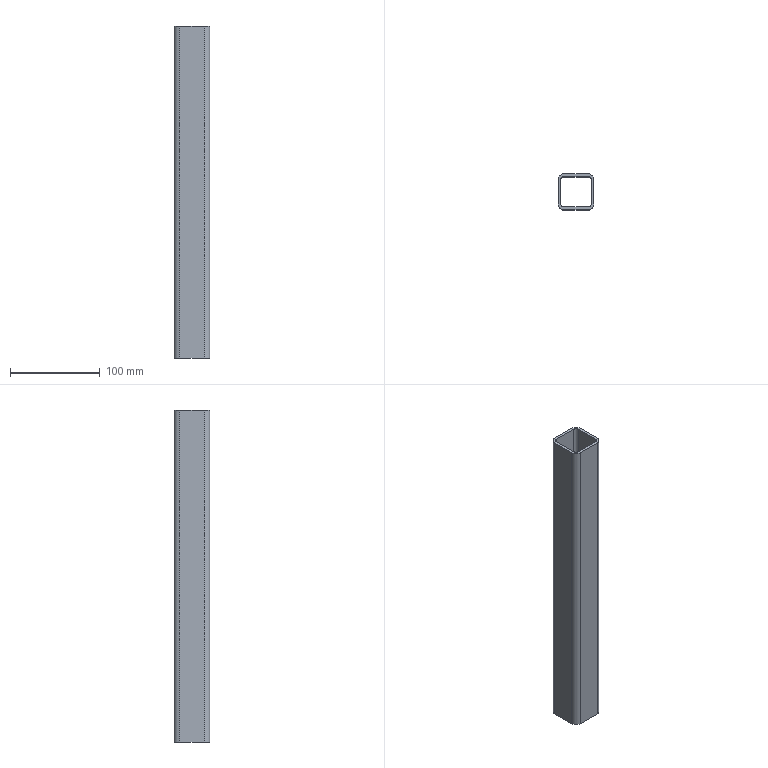Part | STEP file | 2 | 1 solid | 18 faces | box 40 x 40 x 370 mm | volume 154561 mm3 | plane 10 | cylinder 8 | commonest cylinder face diameters 7.2 x4 13.2 x4
STEP:
#1=CARTESIAN_POINT('',(0.,0.,0.));
#2=DIRECTION('',(0.,0.,1.));
#3=DIRECTION('',(1.,0.,0.));
#4=AXIS2_PLACEMENT_3D('',#1,#2,#3);
#5=CARTESIAN_POINT('',(-13.4,-17.,370.));
#6=VERTEX_POINT('',#5);
#7=CARTESIAN_POINT('',(13.4,-17.,370.));
#8=VERTEX_POINT('',#7);
#9=CARTESIAN_POINT('',(6.7,-17.,370.));
#10=DIRECTION('',(1.,0.,0.));
#11=VECTOR('',#10,1.);
#12=LINE('',#9,#11);
#13=CARTESIAN_POINT('',(13.4,-17.,0.));
#14=DIRECTION('',(0.,-1.,0.));
#15=DIRECTION('',(0.,0.,-1.));
#16=AXIS2_PLACEMENT_3D('',#13,#14,#15);
#17=PLANE('',#16);
#18=CARTESIAN_POINT('',(-370.,-6.7));
#19=DIRECTION('',(0.,1.));
#20=VECTOR('',#19,1.);
#21=LINE('',#18,#20);
#22=(GEOMETRIC_REPRESENTATION_CONTEXT(2)PARAMETRIC_REPRESENTATION_CONTEXT()REPRESENTATION_CONTEXT('',''));
#23=DEFINITIONAL_REPRESENTATION('',(#21),#22);
#24=PCURVE('',#17,#23);
#25=CARTESIAN_POINT('',(0.,0.,370.));
#26=DIRECTION('',(0.,0.,1.));
#27=DIRECTION('',(1.,0.,0.));
#28=AXIS2_PLACEMENT_3D('',#25,#26,#27);
#29=PLANE('',#28);
#30=CARTESIAN_POINT('',(6.7,-17.));
#31=DIRECTION('',(1.,0.));
#32=VECTOR('',#31,1.);
#33=LINE('',#30,#32);
#34=(GEOMETRIC_REPRESENTATION_CONTEXT(2)PARAMETRIC_REPRESENTATION_CONTEXT()REPRESENTATION_CONTEXT('',''));
#35=DEFINITIONAL_REPRESENTATION('',(#33),#34);
#36=PCURVE('',#29,#35);
#37=SURFACE_CURVE('',#12,(#24,#36),.PCURVE_S1.);
#38=EDGE_CURVE('',#6,#8,#37,.T.);
#39=ORIENTED_EDGE('',*,*,#38,.T.);
#40=CARTESIAN_POINT('',(13.4,-17.,0.));
#41=VERTEX_POINT('',#40);
#42=CARTESIAN_POINT('',(13.4,-17.,0.));
#43=DIRECTION('',(0.,0.,1.));
#44=VECTOR('',#43,1.);
#45=LINE('',#42,#44);
#46=CARTESIAN_POINT('',(0.,0.));
#47=DIRECTION('',(-1.,0.));
#48=VECTOR('',#47,1.);
#49=LINE('',#46,#48);
#50=(GEOMETRIC_REPRESENTATION_CONTEXT(2)PARAMETRIC_REPRESENTATION_CONTEXT()REPRESENTATION_CONTEXT('',''));
#51=DEFINITIONAL_REPRESENTATION('',(#49),#50);
#52=PCURVE('',#17,#51);
#53=CARTESIAN_POINT('',(13.4,-13.4,0.));
#54=DIRECTION('',(0.,0.,1.));
#55=DIRECTION('',(0.,1.,0.));
#56=AXIS2_PLACEMENT_3D('',#53,#54,#55);
#57=CYLINDRICAL_SURFACE('',#56,3.6);
#58=CARTESIAN_POINT('',(3.142,0.));
#59=DIRECTION('',(0.,1.));
#60=VECTOR('',#59,1.);
#61=LINE('',#58,#60);
#62=(GEOMETRIC_REPRESENTATION_CONTEXT(2)PARAMETRIC_REPRESENTATION_CONTEXT()REPRESENTATION_CONTEXT('',''));
#63=DEFINITIONAL_REPRESENTATION('',(#61),#62);
#64=PCURVE('',#57,#63);
#65=SURFACE_CURVE('',#45,(#52,#64),.PCURVE_S1.);
#66=EDGE_CURVE('',#41,#8,#65,.T.);
#67=ORIENTED_EDGE('',*,*,#66,.F.);
#68=CARTESIAN_POINT('',(-13.4,-17.,0.));
#69=VERTEX_POINT('',#68);
#70=CARTESIAN_POINT('',(6.7,-17.,0.));
#71=DIRECTION('',(1.,0.,0.));
#72=VECTOR('',#71,1.);
#73=LINE('',#70,#72);
#74=CARTESIAN_POINT('',(0.,-6.7));
#75=DIRECTION('',(0.,1.));
#76=VECTOR('',#75,1.);
#77=LINE('',#74,#76);
#78=(GEOMETRIC_REPRESENTATION_CONTEXT(2)PARAMETRIC_REPRESENTATION_CONTEXT()REPRESENTATION_CONTEXT('',''));
#79=DEFINITIONAL_REPRESENTATION('',(#77),#78);
#80=PCURVE('',#17,#79);
#81=CARTESIAN_POINT('',(0.,0.,0.));
#82=DIRECTION('',(0.,0.,1.));
#83=DIRECTION('',(1.,0.,0.));
#84=AXIS2_PLACEMENT_3D('',#81,#82,#83);
#85=PLANE('',#84);
#86=CARTESIAN_POINT('',(6.7,-17.));
#87=DIRECTION('',(1.,0.));
#88=VECTOR('',#87,1.);
#89=LINE('',#86,#88);
#90=(GEOMETRIC_REPRESENTATION_CONTEXT(2)PARAMETRIC_REPRESENTATION_CONTEXT()REPRESENTATION_CONTEXT('',''));
#91=DEFINITIONAL_REPRESENTATION('',(#89),#90);
#92=PCURVE('',#85,#91);
#93=SURFACE_CURVE('',#73,(#80,#92),.PCURVE_S1.);
#94=EDGE_CURVE('',#69,#41,#93,.T.);
#95=ORIENTED_EDGE('',*,*,#94,.F.);
#96=CARTESIAN_POINT('',(-13.4,-17.,0.));
#97=DIRECTION('',(0.,0.,1.));
#98=VECTOR('',#97,1.);
#99=LINE('',#96,#98);
#100=CARTESIAN_POINT('',(0.,-26.8));
#101=DIRECTION('',(-1.,0.));
#102=VECTOR('',#101,1.);
#103=LINE('',#100,#102);
#104=(GEOMETRIC_REPRESENTATION_CONTEXT(2)PARAMETRIC_REPRESENTATION_CONTEXT()REPRESENTATION_CONTEXT('',''));
#105=DEFINITIONAL_REPRESENTATION('',(#103),#104);
#106=PCURVE('',#17,#105);
#107=CARTESIAN_POINT('',(-13.4,-13.4,0.));
#108=DIRECTION('',(0.,0.,1.));
#109=DIRECTION('',(1.,0.,0.));
#110=AXIS2_PLACEMENT_3D('',#107,#108,#109);
#111=CYLINDRICAL_SURFACE('',#110,3.6);
#112=CARTESIAN_POINT('',(4.712,0.));
#113=DIRECTION('',(0.,1.));
#114=VECTOR('',#113,1.);
#115=LINE('',#112,#114);
#116=(GEOMETRIC_REPRESENTATION_CONTEXT(2)PARAMETRIC_REPRESENTATION_CONTEXT()REPRESENTATION_CONTEXT('',''));
#117=DEFINITIONAL_REPRESENTATION('',(#115),#116);
#118=PCURVE('',#111,#117);
#119=SURFACE_CURVE('',#99,(#106,#118),.PCURVE_S1.);
#120=EDGE_CURVE('',#69,#6,#119,.T.);
#121=ORIENTED_EDGE('',*,*,#120,.T.);
#122=EDGE_LOOP('',(#39,#67,#95,#121));
#123=FACE_BOUND('',#122,.T.);
#124=ADVANCED_FACE('',(#123),#17,.F.);
#125=ORIENTED_EDGE('',*,*,#66,.F.);
#126=CARTESIAN_POINT('',(17.,-13.4,0.));
#127=VERTEX_POINT('',#126);
#128=CARTESIAN_POINT('',(13.4,-13.4,0.));
#129=DIRECTION('',(0.,0.,1.));
#130=DIRECTION('',(0.,1.,0.));
#131=AXIS2_PLACEMENT_3D('',#128,#129,#130);
#132=CIRCLE('',#131,3.6);
#133=CARTESIAN_POINT('',(0.,0.));
#134=DIRECTION('',(1.,0.));
#135=VECTOR('',#134,1.);
#136=LINE('',#133,#135);
#137=(GEOMETRIC_REPRESENTATION_CONTEXT(2)PARAMETRIC_REPRESENTATION_CONTEXT()REPRESENTATION_CONTEXT('',''));
#138=DEFINITIONAL_REPRESENTATION('',(#136),#137);
#139=PCURVE('',#57,#138);
#140=CARTESIAN_POINT('',(13.4,-13.4));
#141=DIRECTION('',(0.,1.));
#142=AXIS2_PLACEMENT_2D('',#140,#141);
#143=CIRCLE('',#142,3.6);
#144=(GEOMETRIC_REPRESENTATION_CONTEXT(2)PARAMETRIC_REPRESENTATION_CONTEXT()REPRESENTATION_CONTEXT('',''));
#145=DEFINITIONAL_REPRESENTATION('',(#143),#144);
#146=PCURVE('',#85,#145);
#147=SURFACE_CURVE('',#132,(#139,#146),.PCURVE_S1.);
#148=EDGE_CURVE('',#41,#127,#147,.T.);
#149=ORIENTED_EDGE('',*,*,#148,.T.);
#150=CARTESIAN_POINT('',(17.,-13.4,370.));
#151=VERTEX_POINT('',#150);
#152=CARTESIAN_POINT('',(17.,-13.4,0.));
#153=DIRECTION('',(0.,0.,1.));
#154=VECTOR('',#153,1.);
#155=LINE('',#152,#154);
#156=CARTESIAN_POINT('',(4.712,0.));
#157=DIRECTION('',(0.,1.));
#158=VECTOR('',#157,1.);
#159=LINE('',#156,#158);
#160=(GEOMETRIC_REPRESENTATION_CONTEXT(2)PARAMETRIC_REPRESENTATION_CONTEXT()REPRESENTATION_CONTEXT('',''));
#161=DEFINITIONAL_REPRESENTATION('',(#159),#160);
#162=PCURVE('',#57,#161);
#163=CARTESIAN_POINT('',(17.,13.4,0.));
#164=DIRECTION('',(1.,0.,0.));
#165=DIRECTION('',(0.,0.,-1.));
#166=AXIS2_PLACEMENT_3D('',#163,#164,#165);
#167=PLANE('',#166);
#168=CARTESIAN_POINT('',(0.,-26.8));
#169=DIRECTION('',(-1.,0.));
#170=VECTOR('',#169,1.);
#171=LINE('',#168,#170);
#172=(GEOMETRIC_REPRESENTATION_CONTEXT(2)PARAMETRIC_REPRESENTATION_CONTEXT()REPRESENTATION_CONTEXT('',''));
#173=DEFINITIONAL_REPRESENTATION('',(#171),#172);
#174=PCURVE('',#167,#173);
#175=SURFACE_CURVE('',#155,(#162,#174),.PCURVE_S1.);
#176=EDGE_CURVE('',#127,#151,#175,.T.);
#177=ORIENTED_EDGE('',*,*,#176,.T.);
#178=CARTESIAN_POINT('',(13.4,-13.4,370.));
#179=DIRECTION('',(0.,0.,1.));
#180=DIRECTION('',(0.,1.,0.));
#181=AXIS2_PLACEMENT_3D('',#178,#179,#180);
#182=CIRCLE('',#181,3.6);
#183=CARTESIAN_POINT('',(0.,370.));
#184=DIRECTION('',(1.,0.));
#185=VECTOR('',#184,1.);
#186=LINE('',#183,#185);
#187=(GEOMETRIC_REPRESENTATION_CONTEXT(2)PARAMETRIC_REPRESENTATION_CONTEXT()REPRESENTATION_CONTEXT('',''));
#188=DEFINITIONAL_REPRESENTATION('',(#186),#187);
#189=PCURVE('',#57,#188);
#190=CARTESIAN_POINT('',(13.4,-13.4));
#191=DIRECTION('',(0.,1.));
#192=AXIS2_PLACEMENT_2D('',#190,#191);
#193=CIRCLE('',#192,3.6);
#194=(GEOMETRIC_REPRESENTATION_CONTEXT(2)PARAMETRIC_REPRESENTATION_CONTEXT()REPRESENTATION_CONTEXT('',''));
#195=DEFINITIONAL_REPRESENTATION('',(#193),#194);
#196=PCURVE('',#29,#195);
#197=SURFACE_CURVE('',#182,(#189,#196),.PCURVE_S1.);
#198=EDGE_CURVE('',#8,#151,#197,.T.);
#199=ORIENTED_EDGE('',*,*,#198,.F.);
#200=EDGE_LOOP('',(#125,#149,#177,#199));
#201=FACE_BOUND('',#200,.F.);
#202=ADVANCED_FACE('',(#201),#57,.F.);
#203=CARTESIAN_POINT('',(17.,13.4,370.));
#204=VERTEX_POINT('',#203);
#205=CARTESIAN_POINT('',(17.,6.7,370.));
#206=DIRECTION('',(0.,1.,0.));
#207=VECTOR('',#206,1.);
#208=LINE('',#205,#207);
#209=CARTESIAN_POINT('',(-370.,-6.7));
#210=DIRECTION('',(0.,1.));
#211=VECTOR('',#210,1.);
#212=LINE('',#209,#211);
#213=(GEOMETRIC_REPRESENTATION_CONTEXT(2)PARAMETRIC_REPRESENTATION_CONTEXT()REPRESENTATION_CONTEXT('',''));
#214=DEFINITIONAL_REPRESENTATION('',(#212),#213);
#215=PCURVE('',#167,#214);
#216=CARTESIAN_POINT('',(17.,6.7));
#217=DIRECTION('',(0.,1.));
#218=VECTOR('',#217,1.);
#219=LINE('',#216,#218);
#220=(GEOMETRIC_REPRESENTATION_CONTEXT(2)PARAMETRIC_REPRESENTATION_CONTEXT()REPRESENTATION_CONTEXT('',''));
#221=DEFINITIONAL_REPRESENTATION('',(#219),#220);
#222=PCURVE('',#29,#221);
#223=SURFACE_CURVE('',#208,(#215,#222),.PCURVE_S1.);
#224=EDGE_CURVE('',#151,#204,#223,.T.);
#225=ORIENTED_EDGE('',*,*,#224,.T.);
#226=CARTESIAN_POINT('',(17.,13.4,0.));
#227=VERTEX_POINT('',#226);
#228=CARTESIAN_POINT('',(17.,13.4,0.));
#229=DIRECTION('',(0.,0.,1.));
#230=VECTOR('',#229,1.);
#231=LINE('',#228,#230);
#232=CARTESIAN_POINT('',(0.,0.));
#233=DIRECTION('',(-1.,0.));
#234=VECTOR('',#233,1.);
#235=LINE('',#232,#234);
#236=(GEOMETRIC_REPRESENTATION_CONTEXT(2)PARAMETRIC_REPRESENTATION_CONTEXT()REPRESENTATION_CONTEXT('',''));
#237=DEFINITIONAL_REPRESENTATION('',(#235),#236);
#238=PCURVE('',#167,#237);
#239=CARTESIAN_POINT('',(13.4,13.4,0.));
#240=DIRECTION('',(0.,0.,1.));
#241=DIRECTION('',(-1.,0.,0.));
#242=AXIS2_PLACEMENT_3D('',#239,#240,#241);
#243=CYLINDRICAL_SURFACE('',#242,3.6);
#244=CARTESIAN_POINT('',(3.142,0.));
#245=DIRECTION('',(0.,1.));
#246=VECTOR('',#245,1.);
#247=LINE('',#244,#246);
#248=(GEOMETRIC_REPRESENTATION_CONTEXT(2)PARAMETRIC_REPRESENTATION_CONTEXT()REPRESENTATION_CONTEXT('',''));
#249=DEFINITIONAL_REPRESENTATION('',(#247),#248);
#250=PCURVE('',#243,#249);
#251=SURFACE_CURVE('',#231,(#238,#250),.PCURVE_S1.);
#252=EDGE_CURVE('',#227,#204,#251,.T.);
#253=ORIENTED_EDGE('',*,*,#252,.F.);
#254=CARTESIAN_POINT('',(17.,6.7,0.));
#255=DIRECTION('',(0.,1.,0.));
#256=VECTOR('',#255,1.);
#257=LINE('',#254,#256);
#258=CARTESIAN_POINT('',(0.,-6.7));
#259=DIRECTION('',(0.,1.));
#260=VECTOR('',#259,1.);
#261=LINE('',#258,#260);
#262=(GEOMETRIC_REPRESENTATION_CONTEXT(2)PARAMETRIC_REPRESENTATION_CONTEXT()REPRESENTATION_CONTEXT('',''));
#263=DEFINITIONAL_REPRESENTATION('',(#261),#262);
#264=PCURVE('',#167,#263);
#265=CARTESIAN_POINT('',(17.,6.7));
#266=DIRECTION('',(0.,1.));
#267=VECTOR('',#266,1.);
#268=LINE('',#265,#267);
#269=(GEOMETRIC_REPRESENTATION_CONTEXT(2)PARAMETRIC_REPRESENTATION_CONTEXT()REPRESENTATION_CONTEXT('',''));
#270=DEFINITIONAL_REPRESENTATION('',(#268),#269);
#271=PCURVE('',#85,#270);
#272=SURFACE_CURVE('',#257,(#264,#271),.PCURVE_S1.);
#273=EDGE_CURVE('',#127,#227,#272,.T.);
#274=ORIENTED_EDGE('',*,*,#273,.F.);
#275=ORIENTED_EDGE('',*,*,#176,.T.);
#276=EDGE_LOOP('',(#225,#253,#274,#275));
#277=FACE_BOUND('',#276,.T.);
#278=ADVANCED_FACE('',(#277),#167,.F.);
#279=ORIENTED_EDGE('',*,*,#252,.F.);
#280=CARTESIAN_POINT('',(13.4,17.,0.));
#281=VERTEX_POINT('',#280);
#282=CARTESIAN_POINT('',(13.4,13.4,0.));
#283=DIRECTION('',(0.,0.,1.));
#284=DIRECTION('',(-1.,0.,0.));
#285=AXIS2_PLACEMENT_3D('',#282,#283,#284);
#286=CIRCLE('',#285,3.6);
#287=CARTESIAN_POINT('',(0.,0.));
#288=DIRECTION('',(1.,0.));
#289=VECTOR('',#288,1.);
#290=LINE('',#287,#289);
#291=(GEOMETRIC_REPRESENTATION_CONTEXT(2)PARAMETRIC_REPRESENTATION_CONTEXT()REPRESENTATION_CONTEXT('',''));
#292=DEFINITIONAL_REPRESENTATION('',(#290),#291);
#293=PCURVE('',#243,#292);
#294=CARTESIAN_POINT('',(13.4,13.4));
#295=DIRECTION('',(-1.,0.));
#296=AXIS2_PLACEMENT_2D('',#294,#295);
#297=CIRCLE('',#296,3.6);
#298=(GEOMETRIC_REPRESENTATION_CONTEXT(2)PARAMETRIC_REPRESENTATION_CONTEXT()REPRESENTATION_CONTEXT('',''));
#299=DEFINITIONAL_REPRESENTATION('',(#297),#298);
#300=PCURVE('',#85,#299);
#301=SURFACE_CURVE('',#286,(#293,#300),.PCURVE_S1.);
#302=EDGE_CURVE('',#227,#281,#301,.T.);
#303=ORIENTED_EDGE('',*,*,#302,.T.);
#304=CARTESIAN_POINT('',(13.4,17.,370.));
#305=VERTEX_POINT('',#304);
#306=CARTESIAN_POINT('',(13.4,17.,0.));
#307=DIRECTION('',(0.,0.,1.));
#308=VECTOR('',#307,1.);
#309=LINE('',#306,#308);
#310=CARTESIAN_POINT('',(4.712,0.));
#311=DIRECTION('',(0.,1.));
#312=VECTOR('',#311,1.);
#313=LINE('',#310,#312);
#314=(GEOMETRIC_REPRESENTATION_CONTEXT(2)PARAMETRIC_REPRESENTATION_CONTEXT()REPRESENTATION_CONTEXT('',''));
#315=DEFINITIONAL_REPRESENTATION('',(#313),#314);
#316=PCURVE('',#243,#315);
#317=CARTESIAN_POINT('',(-13.4,17.,0.));
#318=DIRECTION('',(0.,1.,0.));
#319=DIRECTION('',(0.,0.,1.));
#320=AXIS2_PLACEMENT_3D('',#317,#318,#319);
#321=PLANE('',#320);
#322=CARTESIAN_POINT('',(0.,26.8));
#323=DIRECTION('',(1.,0.));
#324=VECTOR('',#323,1.);
#325=LINE('',#322,#324);
#326=(GEOMETRIC_REPRESENTATION_CONTEXT(2)PARAMETRIC_REPRESENTATION_CONTEXT()REPRESENTATION_CONTEXT('',''));
#327=DEFINITIONAL_REPRESENTATION('',(#325),#326);
#328=PCURVE('',#321,#327);
#329=SURFACE_CURVE('',#309,(#316,#328),.PCURVE_S1.);
#330=EDGE_CURVE('',#281,#305,#329,.T.);
#331=ORIENTED_EDGE('',*,*,#330,.T.);
#332=CARTESIAN_POINT('',(13.4,13.4,370.));
#333=DIRECTION('',(0.,0.,1.));
#334=DIRECTION('',(-1.,0.,0.));
#335=AXIS2_PLACEMENT_3D('',#332,#333,#334);
#336=CIRCLE('',#335,3.6);
#337=CARTESIAN_POINT('',(0.,370.));
#338=DIRECTION('',(1.,0.));
#339=VECTOR('',#338,1.);
#340=LINE('',#337,#339);
#341=(GEOMETRIC_REPRESENTATION_CONTEXT(2)PARAMETRIC_REPRESENTATION_CONTEXT()REPRESENTATION_CONTEXT('',''));
#342=DEFINITIONAL_REPRESENTATION('',(#340),#341);
#343=PCURVE('',#243,#342);
#344=CARTESIAN_POINT('',(13.4,13.4));
#345=DIRECTION('',(-1.,0.));
#346=AXIS2_PLACEMENT_2D('',#344,#345);
#347=CIRCLE('',#346,3.6);
#348=(GEOMETRIC_REPRESENTATION_CONTEXT(2)PARAMETRIC_REPRESENTATION_CONTEXT()REPRESENTATION_CONTEXT('',''));
#349=DEFINITIONAL_REPRESENTATION('',(#347),#348);
#350=PCURVE('',#29,#349);
#351=SURFACE_CURVE('',#336,(#343,#350),.PCURVE_S1.);
#352=EDGE_CURVE('',#204,#305,#351,.T.);
#353=ORIENTED_EDGE('',*,*,#352,.F.);
#354=EDGE_LOOP('',(#279,#303,#331,#353));
#355=FACE_BOUND('',#354,.F.);
#356=ADVANCED_FACE('',(#355),#243,.F.);
#357=CARTESIAN_POINT('',(20.,13.4,370.));
#358=VERTEX_POINT('',#357);
#359=CARTESIAN_POINT('',(20.,-13.4,370.));
#360=VERTEX_POINT('',#359);
#361=CARTESIAN_POINT('',(20.,6.7,370.));
#362=DIRECTION('',(0.,-1.,0.));
#363=VECTOR('',#362,1.);
#364=LINE('',#361,#363);
#365=CARTESIAN_POINT('',(20.,13.4,0.));
#366=DIRECTION('',(1.,0.,0.));
#367=DIRECTION('',(0.,0.,-1.));
#368=AXIS2_PLACEMENT_3D('',#365,#366,#367);
#369=PLANE('',#368);
#370=CARTESIAN_POINT('',(-370.,-6.7));
#371=DIRECTION('',(0.,-1.));
#372=VECTOR('',#371,1.);
#373=LINE('',#370,#372);
#374=(GEOMETRIC_REPRESENTATION_CONTEXT(2)PARAMETRIC_REPRESENTATION_CONTEXT()REPRESENTATION_CONTEXT('',''));
#375=DEFINITIONAL_REPRESENTATION('',(#373),#374);
#376=PCURVE('',#369,#375);
#377=CARTESIAN_POINT('',(20.,6.7));
#378=DIRECTION('',(0.,-1.));
#379=VECTOR('',#378,1.);
#380=LINE('',#377,#379);
#381=(GEOMETRIC_REPRESENTATION_CONTEXT(2)PARAMETRIC_REPRESENTATION_CONTEXT()REPRESENTATION_CONTEXT('',''));
#382=DEFINITIONAL_REPRESENTATION('',(#380),#381);
#383=PCURVE('',#29,#382);
#384=SURFACE_CURVE('',#364,(#376,#383),.PCURVE_S1.);
#385=EDGE_CURVE('',#358,#360,#384,.T.);
#386=ORIENTED_EDGE('',*,*,#385,.T.);
#387=CARTESIAN_POINT('',(20.,-13.4,0.));
#388=VERTEX_POINT('',#387);
#389=CARTESIAN_POINT('',(20.,-13.4,0.));
#390=DIRECTION('',(0.,0.,1.));
#391=VECTOR('',#390,1.);
#392=LINE('',#389,#391);
#393=CARTESIAN_POINT('',(0.,-26.8));
#394=DIRECTION('',(-1.,0.));
#395=VECTOR('',#394,1.);
#396=LINE('',#393,#395);
#397=(GEOMETRIC_REPRESENTATION_CONTEXT(2)PARAMETRIC_REPRESENTATION_CONTEXT()REPRESENTATION_CONTEXT('',''));
#398=DEFINITIONAL_REPRESENTATION('',(#396),#397);
#399=PCURVE('',#369,#398);
#400=CARTESIAN_POINT('',(13.4,-13.4,0.));
#401=DIRECTION('',(0.,0.,1.));
#402=DIRECTION('',(0.,1.,0.));
#403=AXIS2_PLACEMENT_3D('',#400,#401,#402);
#404=CYLINDRICAL_SURFACE('',#403,6.6);
#405=CARTESIAN_POINT('',(4.712,0.));
#406=DIRECTION('',(0.,1.));
#407=VECTOR('',#406,1.);
#408=LINE('',#405,#407);
#409=(GEOMETRIC_REPRESENTATION_CONTEXT(2)PARAMETRIC_REPRESENTATION_CONTEXT()REPRESENTATION_CONTEXT('',''));
#410=DEFINITIONAL_REPRESENTATION('',(#408),#409);
#411=PCURVE('',#404,#410);
#412=SURFACE_CURVE('',#392,(#399,#411),.PCURVE_S1.);
#413=EDGE_CURVE('',#388,#360,#412,.T.);
#414=ORIENTED_EDGE('',*,*,#413,.F.);
#415=CARTESIAN_POINT('',(20.,13.4,0.));
#416=VERTEX_POINT('',#415);
#417=CARTESIAN_POINT('',(20.,6.7,0.));
#418=DIRECTION('',(0.,-1.,0.));
#419=VECTOR('',#418,1.);
#420=LINE('',#417,#419);
#421=CARTESIAN_POINT('',(0.,-6.7));
#422=DIRECTION('',(0.,-1.));
#423=VECTOR('',#422,1.);
#424=LINE('',#421,#423);
#425=(GEOMETRIC_REPRESENTATION_CONTEXT(2)PARAMETRIC_REPRESENTATION_CONTEXT()REPRESENTATION_CONTEXT('',''));
#426=DEFINITIONAL_REPRESENTATION('',(#424),#425);
#427=PCURVE('',#369,#426);
#428=CARTESIAN_POINT('',(20.,6.7));
#429=DIRECTION('',(0.,-1.));
#430=VECTOR('',#429,1.);
#431=LINE('',#428,#430);
#432=(GEOMETRIC_REPRESENTATION_CONTEXT(2)PARAMETRIC_REPRESENTATION_CONTEXT()REPRESENTATION_CONTEXT('',''));
#433=DEFINITIONAL_REPRESENTATION('',(#431),#432);
#434=PCURVE('',#85,#433);
#435=SURFACE_CURVE('',#420,(#427,#434),.PCURVE_S1.);
#436=EDGE_CURVE('',#416,#388,#435,.T.);
#437=ORIENTED_EDGE('',*,*,#436,.F.);
#438=CARTESIAN_POINT('',(20.,13.4,0.));
#439=DIRECTION('',(0.,0.,1.));
#440=VECTOR('',#439,1.);
#441=LINE('',#438,#440);
#442=CARTESIAN_POINT('',(0.,0.));
#443=DIRECTION('',(-1.,0.));
#444=VECTOR('',#443,1.);
#445=LINE('',#442,#444);
#446=(GEOMETRIC_REPRESENTATION_CONTEXT(2)PARAMETRIC_REPRESENTATION_CONTEXT()REPRESENTATION_CONTEXT('',''));
#447=DEFINITIONAL_REPRESENTATION('',(#445),#446);
#448=PCURVE('',#369,#447);
#449=CARTESIAN_POINT('',(13.4,13.4,0.));
#450=DIRECTION('',(0.,0.,1.));
#451=DIRECTION('',(-1.,0.,0.));
#452=AXIS2_PLACEMENT_3D('',#449,#450,#451);
#453=CYLINDRICAL_SURFACE('',#452,6.6);
#454=CARTESIAN_POINT('',(3.142,0.));
#455=DIRECTION('',(0.,1.));
#456=VECTOR('',#455,1.);
#457=LINE('',#454,#456);
#458=(GEOMETRIC_REPRESENTATION_CONTEXT(2)PARAMETRIC_REPRESENTATION_CONTEXT()REPRESENTATION_CONTEXT('',''));
#459=DEFINITIONAL_REPRESENTATION('',(#457),#458);
#460=PCURVE('',#453,#459);
#461=SURFACE_CURVE('',#441,(#448,#460),.PCURVE_S1.);
#462=EDGE_CURVE('',#416,#358,#461,.T.);
#463=ORIENTED_EDGE('',*,*,#462,.T.);
#464=EDGE_LOOP('',(#386,#414,#437,#463));
#465=FACE_BOUND('',#464,.T.);
#466=ADVANCED_FACE('',(#465),#369,.T.);
#467=CARTESIAN_POINT('',(13.4,-20.,370.));
#468=VERTEX_POINT('',#467);
#469=CARTESIAN_POINT('',(13.4,-13.4,370.));
#470=DIRECTION('',(0.,0.,-1.));
#471=DIRECTION('',(0.,1.,0.));
#472=AXIS2_PLACEMENT_3D('',#469,#470,#471);
#473=CIRCLE('',#472,6.6);
#474=CARTESIAN_POINT('',(6.283,370.));
#475=DIRECTION('',(-1.,0.));
#476=VECTOR('',#475,1.);
#477=LINE('',#474,#476);
#478=(GEOMETRIC_REPRESENTATION_CONTEXT(2)PARAMETRIC_REPRESENTATION_CONTEXT()REPRESENTATION_CONTEXT('',''));
#479=DEFINITIONAL_REPRESENTATION('',(#477),#478);
#480=PCURVE('',#404,#479);
#481=CARTESIAN_POINT('',(13.4,-6.8));
#482=CARTESIAN_POINT('',(24.832,-6.8));
#483=CARTESIAN_POINT('',(19.116,-16.7));
#484=CARTESIAN_POINT('',(13.4,-26.6));
#485=CARTESIAN_POINT('',(7.684,-16.7));
#486=CARTESIAN_POINT('',(1.968,-6.8));
#487=CARTESIAN_POINT('',(13.4,-6.8));
#488=(BOUNDED_CURVE()B_SPLINE_CURVE(2,(#481,#482,#483,#484,#485,#486,#487),.UNSPECIFIED.,.T.,.F.)B_SPLINE_CURVE_WITH_KNOTS((1,2,2,2,2,1),(-2.094,0.,2.094,4.189,6.283,8.378),.UNSPECIFIED.)CURVE()GEOMETRIC_REPRESENTATION_ITEM()RATIONAL_B_SPLINE_CURVE((1.,0.5,1.,0.5,1.,0.5,1.))REPRESENTATION_ITEM(''));
#489=(GEOMETRIC_REPRESENTATION_CONTEXT(2)PARAMETRIC_REPRESENTATION_CONTEXT()REPRESENTATION_CONTEXT('',''));
#490=DEFINITIONAL_REPRESENTATION('',(#488),#489);
#491=PCURVE('',#29,#490);
#492=SURFACE_CURVE('',#473,(#480,#491),.PCURVE_S1.);
#493=EDGE_CURVE('',#360,#468,#492,.T.);
#494=ORIENTED_EDGE('',*,*,#493,.T.);
#495=CARTESIAN_POINT('',(13.4,-20.,0.));
#496=VERTEX_POINT('',#495);
#497=CARTESIAN_POINT('',(13.4,-20.,0.));
#498=DIRECTION('',(0.,0.,1.));
#499=VECTOR('',#498,1.);
#500=LINE('',#497,#499);
#501=CARTESIAN_POINT('',(3.142,0.));
#502=DIRECTION('',(0.,1.));
#503=VECTOR('',#502,1.);
#504=LINE('',#501,#503);
#505=(GEOMETRIC_REPRESENTATION_CONTEXT(2)PARAMETRIC_REPRESENTATION_CONTEXT()REPRESENTATION_CONTEXT('',''));
#506=DEFINITIONAL_REPRESENTATION('',(#504),#505);
#507=PCURVE('',#404,#506);
#508=CARTESIAN_POINT('',(13.4,-20.,0.));
#509=DIRECTION('',(0.,-1.,0.));
#510=DIRECTION('',(0.,0.,-1.));
#511=AXIS2_PLACEMENT_3D('',#508,#509,#510);
#512=PLANE('',#511);
#513=CARTESIAN_POINT('',(0.,0.));
#514=DIRECTION('',(-1.,0.));
#515=VECTOR('',#514,1.);
#516=LINE('',#513,#515);
#517=(GEOMETRIC_REPRESENTATION_CONTEXT(2)PARAMETRIC_REPRESENTATION_CONTEXT()REPRESENTATION_CONTEXT('',''));
#518=DEFINITIONAL_REPRESENTATION('',(#516),#517);
#519=PCURVE('',#512,#518);
#520=SURFACE_CURVE('',#500,(#507,#519),.PCURVE_S1.);
#521=EDGE_CURVE('',#496,#468,#520,.T.);
#522=ORIENTED_EDGE('',*,*,#521,.F.);
#523=CARTESIAN_POINT('',(13.4,-13.4,0.));
#524=DIRECTION('',(0.,0.,-1.));
#525=DIRECTION('',(0.,1.,0.));
#526=AXIS2_PLACEMENT_3D('',#523,#524,#525);
#527=CIRCLE('',#526,6.6);
#528=CARTESIAN_POINT('',(6.283,0.));
#529=DIRECTION('',(-1.,0.));
#530=VECTOR('',#529,1.);
#531=LINE('',#528,#530);
#532=(GEOMETRIC_REPRESENTATION_CONTEXT(2)PARAMETRIC_REPRESENTATION_CONTEXT()REPRESENTATION_CONTEXT('',''));
#533=DEFINITIONAL_REPRESENTATION('',(#531),#532);
#534=PCURVE('',#404,#533);
#535=CARTESIAN_POINT('',(13.4,-6.8));
#536=CARTESIAN_POINT('',(24.832,-6.8));
#537=CARTESIAN_POINT('',(19.116,-16.7));
#538=CARTESIAN_POINT('',(13.4,-26.6));
#539=CARTESIAN_POINT('',(7.684,-16.7));
#540=CARTESIAN_POINT('',(1.968,-6.8));
#541=CARTESIAN_POINT('',(13.4,-6.8));
#542=(BOUNDED_CURVE()B_SPLINE_CURVE(2,(#535,#536,#537,#538,#539,#540,#541),.UNSPECIFIED.,.T.,.F.)B_SPLINE_CURVE_WITH_KNOTS((1,2,2,2,2,1),(-2.094,0.,2.094,4.189,6.283,8.378),.UNSPECIFIED.)CURVE()GEOMETRIC_REPRESENTATION_ITEM()RATIONAL_B_SPLINE_CURVE((1.,0.5,1.,0.5,1.,0.5,1.))REPRESENTATION_ITEM(''));
#543=(GEOMETRIC_REPRESENTATION_CONTEXT(2)PARAMETRIC_REPRESENTATION_CONTEXT()REPRESENTATION_CONTEXT('',''));
#544=DEFINITIONAL_REPRESENTATION('',(#542),#543);
#545=PCURVE('',#85,#544);
#546=SURFACE_CURVE('',#527,(#534,#545),.PCURVE_S1.);
#547=EDGE_CURVE('',#388,#496,#546,.T.);
#548=ORIENTED_EDGE('',*,*,#547,.F.);
#549=ORIENTED_EDGE('',*,*,#413,.T.);
#550=EDGE_LOOP('',(#494,#522,#548,#549));
#551=FACE_BOUND('',#550,.T.);
#552=ADVANCED_FACE('',(#551),#404,.T.);
#553=CARTESIAN_POINT('',(-13.4,-20.,370.));
#554=VERTEX_POINT('',#553);
#555=CARTESIAN_POINT('',(6.7,-20.,370.));
#556=DIRECTION('',(-1.,0.,0.));
#557=VECTOR('',#556,1.);
#558=LINE('',#555,#557);
#559=CARTESIAN_POINT('',(-370.,-6.7));
#560=DIRECTION('',(0.,-1.));
#561=VECTOR('',#560,1.);
#562=LINE('',#559,#561);
#563=(GEOMETRIC_REPRESENTATION_CONTEXT(2)PARAMETRIC_REPRESENTATION_CONTEXT()REPRESENTATION_CONTEXT('',''));
#564=DEFINITIONAL_REPRESENTATION('',(#562),#563);
#565=PCURVE('',#512,#564);
#566=CARTESIAN_POINT('',(6.7,-20.));
#567=DIRECTION('',(-1.,0.));
#568=VECTOR('',#567,1.);
#569=LINE('',#566,#568);
#570=(GEOMETRIC_REPRESENTATION_CONTEXT(2)PARAMETRIC_REPRESENTATION_CONTEXT()REPRESENTATION_CONTEXT('',''));
#571=DEFINITIONAL_REPRESENTATION('',(#569),#570);
#572=PCURVE('',#29,#571);
#573=SURFACE_CURVE('',#558,(#565,#572),.PCURVE_S1.);
#574=EDGE_CURVE('',#468,#554,#573,.T.);
#575=ORIENTED_EDGE('',*,*,#574,.T.);
#576=CARTESIAN_POINT('',(-13.4,-20.,0.));
#577=VERTEX_POINT('',#576);
#578=CARTESIAN_POINT('',(-13.4,-20.,0.));
#579=DIRECTION('',(0.,0.,1.));
#580=VECTOR('',#579,1.);
#581=LINE('',#578,#580);
#582=CARTESIAN_POINT('',(0.,-26.8));
#583=DIRECTION('',(-1.,0.));
#584=VECTOR('',#583,1.);
#585=LINE('',#582,#584);
#586=(GEOMETRIC_REPRESENTATION_CONTEXT(2)PARAMETRIC_REPRESENTATION_CONTEXT()REPRESENTATION_CONTEXT('',''));
#587=DEFINITIONAL_REPRESENTATION('',(#585),#586);
#588=PCURVE('',#512,#587);
#589=CARTESIAN_POINT('',(-13.4,-13.4,0.));
#590=DIRECTION('',(0.,0.,1.));
#591=DIRECTION('',(1.,0.,0.));
#592=AXIS2_PLACEMENT_3D('',#589,#590,#591);
#593=CYLINDRICAL_SURFACE('',#592,6.6);
#594=CARTESIAN_POINT('',(4.712,0.));
#595=DIRECTION('',(0.,1.));
#596=VECTOR('',#595,1.);
#597=LINE('',#594,#596);
#598=(GEOMETRIC_REPRESENTATION_CONTEXT(2)PARAMETRIC_REPRESENTATION_CONTEXT()REPRESENTATION_CONTEXT('',''));
#599=DEFINITIONAL_REPRESENTATION('',(#597),#598);
#600=PCURVE('',#593,#599);
#601=SURFACE_CURVE('',#581,(#588,#600),.PCURVE_S1.);
#602=EDGE_CURVE('',#577,#554,#601,.T.);
#603=ORIENTED_EDGE('',*,*,#602,.F.);
#604=CARTESIAN_POINT('',(6.7,-20.,0.));
#605=DIRECTION('',(-1.,0.,0.));
#606=VECTOR('',#605,1.);
#607=LINE('',#604,#606);
#608=CARTESIAN_POINT('',(0.,-6.7));
#609=DIRECTION('',(0.,-1.));
#610=VECTOR('',#609,1.);
#611=LINE('',#608,#610);
#612=(GEOMETRIC_REPRESENTATION_CONTEXT(2)PARAMETRIC_REPRESENTATION_CONTEXT()REPRESENTATION_CONTEXT('',''));
#613=DEFINITIONAL_REPRESENTATION('',(#611),#612);
#614=PCURVE('',#512,#613);
#615=CARTESIAN_POINT('',(6.7,-20.));
#616=DIRECTION('',(-1.,0.));
#617=VECTOR('',#616,1.);
#618=LINE('',#615,#617);
#619=(GEOMETRIC_REPRESENTATION_CONTEXT(2)PARAMETRIC_REPRESENTATION_CONTEXT()REPRESENTATION_CONTEXT('',''));
#620=DEFINITIONAL_REPRESENTATION('',(#618),#619);
#621=PCURVE('',#85,#620);
#622=SURFACE_CURVE('',#607,(#614,#621),.PCURVE_S1.);
#623=EDGE_CURVE('',#496,#577,#622,.T.);
#624=ORIENTED_EDGE('',*,*,#623,.F.);
#625=ORIENTED_EDGE('',*,*,#521,.T.);
#626=EDGE_LOOP('',(#575,#603,#624,#625));
#627=FACE_BOUND('',#626,.T.);
#628=ADVANCED_FACE('',(#627),#512,.T.);
#629=CARTESIAN_POINT('',(-20.,-13.4,370.));
#630=VERTEX_POINT('',#629);
#631=CARTESIAN_POINT('',(-13.4,-13.4,370.));
#632=DIRECTION('',(0.,0.,-1.));
#633=DIRECTION('',(1.,0.,0.));
#634=AXIS2_PLACEMENT_3D('',#631,#632,#633);
#635=CIRCLE('',#634,6.6);
#636=CARTESIAN_POINT('',(6.283,370.));
#637=DIRECTION('',(-1.,0.));
#638=VECTOR('',#637,1.);
#639=LINE('',#636,#638);
#640=(GEOMETRIC_REPRESENTATION_CONTEXT(2)PARAMETRIC_REPRESENTATION_CONTEXT()REPRESENTATION_CONTEXT('',''));
#641=DEFINITIONAL_REPRESENTATION('',(#639),#640);
#642=PCURVE('',#593,#641);
#643=CARTESIAN_POINT('',(-6.8,-13.4));
#644=CARTESIAN_POINT('',(-6.8,-24.832));
#645=CARTESIAN_POINT('',(-16.7,-19.116));
#646=CARTESIAN_POINT('',(-26.6,-13.4));
#647=CARTESIAN_POINT('',(-16.7,-7.684));
#648=CARTESIAN_POINT('',(-6.8,-1.968));
#649=CARTESIAN_POINT('',(-6.8,-13.4));
#650=(BOUNDED_CURVE()B_SPLINE_CURVE(2,(#643,#644,#645,#646,#647,#648,#649),.UNSPECIFIED.,.T.,.F.)B_SPLINE_CURVE_WITH_KNOTS((1,2,2,2,2,1),(-2.094,0.,2.094,4.189,6.283,8.378),.UNSPECIFIED.)CURVE()GEOMETRIC_REPRESENTATION_ITEM()RATIONAL_B_SPLINE_CURVE((1.,0.5,1.,0.5,1.,0.5,1.))REPRESENTATION_ITEM(''));
#651=(GEOMETRIC_REPRESENTATION_CONTEXT(2)PARAMETRIC_REPRESENTATION_CONTEXT()REPRESENTATION_CONTEXT('',''));
#652=DEFINITIONAL_REPRESENTATION('',(#650),#651);
#653=PCURVE('',#29,#652);
#654=SURFACE_CURVE('',#635,(#642,#653),.PCURVE_S1.);
#655=EDGE_CURVE('',#554,#630,#654,.T.);
#656=ORIENTED_EDGE('',*,*,#655,.T.);
#657=CARTESIAN_POINT('',(-20.,-13.4,0.));
#658=VERTEX_POINT('',#657);
#659=CARTESIAN_POINT('',(-20.,-13.4,0.));
#660=DIRECTION('',(0.,0.,1.));
#661=VECTOR('',#660,1.);
#662=LINE('',#659,#661);
#663=CARTESIAN_POINT('',(3.142,0.));
#664=DIRECTION('',(0.,1.));
#665=VECTOR('',#664,1.);
#666=LINE('',#663,#665);
#667=(GEOMETRIC_REPRESENTATION_CONTEXT(2)PARAMETRIC_REPRESENTATION_CONTEXT()REPRESENTATION_CONTEXT('',''));
#668=DEFINITIONAL_REPRESENTATION('',(#666),#667);
#669=PCURVE('',#593,#668);
#670=CARTESIAN_POINT('',(-20.,-13.4,0.));
#671=DIRECTION('',(-1.,0.,0.));
#672=DIRECTION('',(0.,0.,1.));
#673=AXIS2_PLACEMENT_3D('',#670,#671,#672);
#674=PLANE('',#673);
#675=CARTESIAN_POINT('',(0.,0.));
#676=DIRECTION('',(1.,0.));
#677=VECTOR('',#676,1.);
#678=LINE('',#675,#677);
#679=(GEOMETRIC_REPRESENTATION_CONTEXT(2)PARAMETRIC_REPRESENTATION_CONTEXT()REPRESENTATION_CONTEXT('',''));
#680=DEFINITIONAL_REPRESENTATION('',(#678),#679);
#681=PCURVE('',#674,#680);
#682=SURFACE_CURVE('',#662,(#669,#681),.PCURVE_S1.);
#683=EDGE_CURVE('',#658,#630,#682,.T.);
#684=ORIENTED_EDGE('',*,*,#683,.F.);
#685=CARTESIAN_POINT('',(-13.4,-13.4,0.));
#686=DIRECTION('',(0.,0.,-1.));
#687=DIRECTION('',(1.,0.,0.));
#688=AXIS2_PLACEMENT_3D('',#685,#686,#687);
#689=CIRCLE('',#688,6.6);
#690=CARTESIAN_POINT('',(6.283,0.));
#691=DIRECTION('',(-1.,0.));
#692=VECTOR('',#691,1.);
#693=LINE('',#690,#692);
#694=(GEOMETRIC_REPRESENTATION_CONTEXT(2)PARAMETRIC_REPRESENTATION_CONTEXT()REPRESENTATION_CONTEXT('',''));
#695=DEFINITIONAL_REPRESENTATION('',(#693),#694);
#696=PCURVE('',#593,#695);
#697=CARTESIAN_POINT('',(-6.8,-13.4));
#698=CARTESIAN_POINT('',(-6.8,-24.832));
#699=CARTESIAN_POINT('',(-16.7,-19.116));
#700=CARTESIAN_POINT('',(-26.6,-13.4));
#701=CARTESIAN_POINT('',(-16.7,-7.684));
#702=CARTESIAN_POINT('',(-6.8,-1.968));
#703=CARTESIAN_POINT('',(-6.8,-13.4));
#704=(BOUNDED_CURVE()B_SPLINE_CURVE(2,(#697,#698,#699,#700,#701,#702,#703),.UNSPECIFIED.,.T.,.F.)B_SPLINE_CURVE_WITH_KNOTS((1,2,2,2,2,1),(-2.094,0.,2.094,4.189,6.283,8.378),.UNSPECIFIED.)CURVE()GEOMETRIC_REPRESENTATION_ITEM()RATIONAL_B_SPLINE_CURVE((1.,0.5,1.,0.5,1.,0.5,1.))REPRESENTATION_ITEM(''));
#705=(GEOMETRIC_REPRESENTATION_CONTEXT(2)PARAMETRIC_REPRESENTATION_CONTEXT()REPRESENTATION_CONTEXT('',''));
#706=DEFINITIONAL_REPRESENTATION('',(#704),#705);
#707=PCURVE('',#85,#706);
#708=SURFACE_CURVE('',#689,(#696,#707),.PCURVE_S1.);
#709=EDGE_CURVE('',#577,#658,#708,.T.);
#710=ORIENTED_EDGE('',*,*,#709,.F.);
#711=ORIENTED_EDGE('',*,*,#602,.T.);
#712=EDGE_LOOP('',(#656,#684,#710,#711));
#713=FACE_BOUND('',#712,.T.);
#714=ADVANCED_FACE('',(#713),#593,.T.);
#715=CARTESIAN_POINT('',(-13.4,17.,370.));
#716=VERTEX_POINT('',#715);
#717=CARTESIAN_POINT('',(-6.7,17.,370.));
#718=DIRECTION('',(-1.,0.,0.));
#719=VECTOR('',#718,1.);
#720=LINE('',#717,#719);
#721=CARTESIAN_POINT('',(370.,6.7));
#722=DIRECTION('',(0.,-1.));
#723=VECTOR('',#722,1.);
#724=LINE('',#721,#723);
#725=(GEOMETRIC_REPRESENTATION_CONTEXT(2)PARAMETRIC_REPRESENTATION_CONTEXT()REPRESENTATION_CONTEXT('',''));
#726=DEFINITIONAL_REPRESENTATION('',(#724),#725);
#727=PCURVE('',#321,#726);
#728=CARTESIAN_POINT('',(-6.7,17.));
#729=DIRECTION('',(-1.,0.));
#730=VECTOR('',#729,1.);
#731=LINE('',#728,#730);
#732=(GEOMETRIC_REPRESENTATION_CONTEXT(2)PARAMETRIC_REPRESENTATION_CONTEXT()REPRESENTATION_CONTEXT('',''));
#733=DEFINITIONAL_REPRESENTATION('',(#731),#732);
#734=PCURVE('',#29,#733);
#735=SURFACE_CURVE('',#720,(#727,#734),.PCURVE_S1.);
#736=EDGE_CURVE('',#305,#716,#735,.T.);
#737=ORIENTED_EDGE('',*,*,#736,.T.);
#738=CARTESIAN_POINT('',(-13.4,17.,0.));
#739=VERTEX_POINT('',#738);
#740=CARTESIAN_POINT('',(-13.4,17.,0.));
#741=DIRECTION('',(0.,0.,1.));
#742=VECTOR('',#741,1.);
#743=LINE('',#740,#742);
#744=CARTESIAN_POINT('',(0.,0.));
#745=DIRECTION('',(1.,0.));
#746=VECTOR('',#745,1.);
#747=LINE('',#744,#746);
#748=(GEOMETRIC_REPRESENTATION_CONTEXT(2)PARAMETRIC_REPRESENTATION_CONTEXT()REPRESENTATION_CONTEXT('',''));
#749=DEFINITIONAL_REPRESENTATION('',(#747),#748);
#750=PCURVE('',#321,#749);
#751=CARTESIAN_POINT('',(-13.4,13.4,0.));
#752=DIRECTION('',(0.,0.,1.));
#753=DIRECTION('',(0.,-1.,0.));
#754=AXIS2_PLACEMENT_3D('',#751,#752,#753);
#755=CYLINDRICAL_SURFACE('',#754,3.6);
#756=CARTESIAN_POINT('',(3.142,0.));
#757=DIRECTION('',(0.,1.));
#758=VECTOR('',#757,1.);
#759=LINE('',#756,#758);
#760=(GEOMETRIC_REPRESENTATION_CONTEXT(2)PARAMETRIC_REPRESENTATION_CONTEXT()REPRESENTATION_CONTEXT('',''));
#761=DEFINITIONAL_REPRESENTATION('',(#759),#760);
#762=PCURVE('',#755,#761);
#763=SURFACE_CURVE('',#743,(#750,#762),.PCURVE_S1.);
#764=EDGE_CURVE('',#739,#716,#763,.T.);
#765=ORIENTED_EDGE('',*,*,#764,.F.);
#766=CARTESIAN_POINT('',(-6.7,17.,0.));
#767=DIRECTION('',(-1.,0.,0.));
#768=VECTOR('',#767,1.);
#769=LINE('',#766,#768);
#770=CARTESIAN_POINT('',(0.,6.7));
#771=DIRECTION('',(0.,-1.));
#772=VECTOR('',#771,1.);
#773=LINE('',#770,#772);
#774=(GEOMETRIC_REPRESENTATION_CONTEXT(2)PARAMETRIC_REPRESENTATION_CONTEXT()REPRESENTATION_CONTEXT('',''));
#775=DEFINITIONAL_REPRESENTATION('',(#773),#774);
#776=PCURVE('',#321,#775);
#777=CARTESIAN_POINT('',(-6.7,17.));
#778=DIRECTION('',(-1.,0.));
#779=VECTOR('',#778,1.);
#780=LINE('',#777,#779);
#781=(GEOMETRIC_REPRESENTATION_CONTEXT(2)PARAMETRIC_REPRESENTATION_CONTEXT()REPRESENTATION_CONTEXT('',''));
#782=DEFINITIONAL_REPRESENTATION('',(#780),#781);
#783=PCURVE('',#85,#782);
#784=SURFACE_CURVE('',#769,(#776,#783),.PCURVE_S1.);
#785=EDGE_CURVE('',#281,#739,#784,.T.);
#786=ORIENTED_EDGE('',*,*,#785,.F.);
#787=ORIENTED_EDGE('',*,*,#330,.T.);
#788=EDGE_LOOP('',(#737,#765,#786,#787));
#789=FACE_BOUND('',#788,.T.);
#790=ADVANCED_FACE('',(#789),#321,.F.);
#791=CARTESIAN_POINT('',(-17.,-13.4,0.));
#792=VERTEX_POINT('',#791);
#793=CARTESIAN_POINT('',(-17.,-13.4,370.));
#794=VERTEX_POINT('',#793);
#795=CARTESIAN_POINT('',(-17.,-13.4,0.));
#796=DIRECTION('',(0.,0.,1.));
#797=VECTOR('',#796,1.);
#798=LINE('',#795,#797);
#799=CARTESIAN_POINT('',(3.142,0.));
#800=DIRECTION('',(0.,1.));
#801=VECTOR('',#800,1.);
#802=LINE('',#799,#801);
#803=(GEOMETRIC_REPRESENTATION_CONTEXT(2)PARAMETRIC_REPRESENTATION_CONTEXT()REPRESENTATION_CONTEXT('',''));
#804=DEFINITIONAL_REPRESENTATION('',(#802),#803);
#805=PCURVE('',#111,#804);
#806=CARTESIAN_POINT('',(-17.,-13.4,0.));
#807=DIRECTION('',(-1.,0.,0.));
#808=DIRECTION('',(0.,0.,1.));
#809=AXIS2_PLACEMENT_3D('',#806,#807,#808);
#810=PLANE('',#809);
#811=CARTESIAN_POINT('',(0.,0.));
#812=DIRECTION('',(1.,0.));
#813=VECTOR('',#812,1.);
#814=LINE('',#811,#813);
#815=(GEOMETRIC_REPRESENTATION_CONTEXT(2)PARAMETRIC_REPRESENTATION_CONTEXT()REPRESENTATION_CONTEXT('',''));
#816=DEFINITIONAL_REPRESENTATION('',(#814),#815);
#817=PCURVE('',#810,#816);
#818=SURFACE_CURVE('',#798,(#805,#817),.PCURVE_S1.);
#819=EDGE_CURVE('',#792,#794,#818,.T.);
#820=ORIENTED_EDGE('',*,*,#819,.F.);
#821=CARTESIAN_POINT('',(-13.4,-13.4,0.));
#822=DIRECTION('',(0.,0.,1.));
#823=DIRECTION('',(1.,0.,0.));
#824=AXIS2_PLACEMENT_3D('',#821,#822,#823);
#825=CIRCLE('',#824,3.6);
#826=CARTESIAN_POINT('',(0.,0.));
#827=DIRECTION('',(1.,0.));
#828=VECTOR('',#827,1.);
#829=LINE('',#826,#828);
#830=(GEOMETRIC_REPRESENTATION_CONTEXT(2)PARAMETRIC_REPRESENTATION_CONTEXT()REPRESENTATION_CONTEXT('',''));
#831=DEFINITIONAL_REPRESENTATION('',(#829),#830);
#832=PCURVE('',#111,#831);
#833=CARTESIAN_POINT('',(-13.4,-13.4));
#834=DIRECTION('',(1.,0.));
#835=AXIS2_PLACEMENT_2D('',#833,#834);
#836=CIRCLE('',#835,3.6);
#837=(GEOMETRIC_REPRESENTATION_CONTEXT(2)PARAMETRIC_REPRESENTATION_CONTEXT()REPRESENTATION_CONTEXT('',''));
#838=DEFINITIONAL_REPRESENTATION('',(#836),#837);
#839=PCURVE('',#85,#838);
#840=SURFACE_CURVE('',#825,(#832,#839),.PCURVE_S1.);
#841=EDGE_CURVE('',#792,#69,#840,.T.);
#842=ORIENTED_EDGE('',*,*,#841,.T.);
#843=ORIENTED_EDGE('',*,*,#120,.T.);
#844=CARTESIAN_POINT('',(-13.4,-13.4,370.));
#845=DIRECTION('',(0.,0.,1.));
#846=DIRECTION('',(1.,0.,0.));
#847=AXIS2_PLACEMENT_3D('',#844,#845,#846);
#848=CIRCLE('',#847,3.6);
#849=CARTESIAN_POINT('',(0.,370.));
#850=DIRECTION('',(1.,0.));
#851=VECTOR('',#850,1.);
#852=LINE('',#849,#851);
#853=(GEOMETRIC_REPRESENTATION_CONTEXT(2)PARAMETRIC_REPRESENTATION_CONTEXT()REPRESENTATION_CONTEXT('',''));
#854=DEFINITIONAL_REPRESENTATION('',(#852),#853);
#855=PCURVE('',#111,#854);
#856=CARTESIAN_POINT('',(-13.4,-13.4));
#857=DIRECTION('',(1.,0.));
#858=AXIS2_PLACEMENT_2D('',#856,#857);
#859=CIRCLE('',#858,3.6);
#860=(GEOMETRIC_REPRESENTATION_CONTEXT(2)PARAMETRIC_REPRESENTATION_CONTEXT()REPRESENTATION_CONTEXT('',''));
#861=DEFINITIONAL_REPRESENTATION('',(#859),#860);
#862=PCURVE('',#29,#861);
#863=SURFACE_CURVE('',#848,(#855,#862),.PCURVE_S1.);
#864=EDGE_CURVE('',#794,#6,#863,.T.);
#865=ORIENTED_EDGE('',*,*,#864,.F.);
#866=EDGE_LOOP('',(#820,#842,#843,#865));
#867=FACE_BOUND('',#866,.F.);
#868=ADVANCED_FACE('',(#867),#111,.F.);
#869=CARTESIAN_POINT('',(-17.,13.4,370.));
#870=VERTEX_POINT('',#869);
#871=CARTESIAN_POINT('',(-17.,-6.7,370.));
#872=DIRECTION('',(0.,-1.,0.));
#873=VECTOR('',#872,1.);
#874=LINE('',#871,#873);
#875=CARTESIAN_POINT('',(370.,6.7));
#876=DIRECTION('',(0.,-1.));
#877=VECTOR('',#876,1.);
#878=LINE('',#875,#877);
#879=(GEOMETRIC_REPRESENTATION_CONTEXT(2)PARAMETRIC_REPRESENTATION_CONTEXT()REPRESENTATION_CONTEXT('',''));
#880=DEFINITIONAL_REPRESENTATION('',(#878),#879);
#881=PCURVE('',#810,#880);
#882=CARTESIAN_POINT('',(-17.,-6.7));
#883=DIRECTION('',(0.,-1.));
#884=VECTOR('',#883,1.);
#885=LINE('',#882,#884);
#886=(GEOMETRIC_REPRESENTATION_CONTEXT(2)PARAMETRIC_REPRESENTATION_CONTEXT()REPRESENTATION_CONTEXT('',''));
#887=DEFINITIONAL_REPRESENTATION('',(#885),#886);
#888=PCURVE('',#29,#887);
#889=SURFACE_CURVE('',#874,(#881,#888),.PCURVE_S1.);
#890=EDGE_CURVE('',#870,#794,#889,.T.);
#891=ORIENTED_EDGE('',*,*,#890,.T.);
#892=ORIENTED_EDGE('',*,*,#819,.F.);
#893=CARTESIAN_POINT('',(-17.,13.4,0.));
#894=VERTEX_POINT('',#893);
#895=CARTESIAN_POINT('',(-17.,-6.7,0.));
#896=DIRECTION('',(0.,-1.,0.));
#897=VECTOR('',#896,1.);
#898=LINE('',#895,#897);
#899=CARTESIAN_POINT('',(0.,6.7));
#900=DIRECTION('',(0.,-1.));
#901=VECTOR('',#900,1.);
#902=LINE('',#899,#901);
#903=(GEOMETRIC_REPRESENTATION_CONTEXT(2)PARAMETRIC_REPRESENTATION_CONTEXT()REPRESENTATION_CONTEXT('',''));
#904=DEFINITIONAL_REPRESENTATION('',(#902),#903);
#905=PCURVE('',#810,#904);
#906=CARTESIAN_POINT('',(-17.,-6.7));
#907=DIRECTION('',(0.,-1.));
#908=VECTOR('',#907,1.);
#909=LINE('',#906,#908);
#910=(GEOMETRIC_REPRESENTATION_CONTEXT(2)PARAMETRIC_REPRESENTATION_CONTEXT()REPRESENTATION_CONTEXT('',''));
#911=DEFINITIONAL_REPRESENTATION('',(#909),#910);
#912=PCURVE('',#85,#911);
#913=SURFACE_CURVE('',#898,(#905,#912),.PCURVE_S1.);
#914=EDGE_CURVE('',#894,#792,#913,.T.);
#915=ORIENTED_EDGE('',*,*,#914,.F.);
#916=CARTESIAN_POINT('',(-17.,13.4,0.));
#917=DIRECTION('',(0.,0.,1.));
#918=VECTOR('',#917,1.);
#919=LINE('',#916,#918);
#920=CARTESIAN_POINT('',(0.,26.8));
#921=DIRECTION('',(1.,0.));
#922=VECTOR('',#921,1.);
#923=LINE('',#920,#922);
#924=(GEOMETRIC_REPRESENTATION_CONTEXT(2)PARAMETRIC_REPRESENTATION_CONTEXT()REPRESENTATION_CONTEXT('',''));
#925=DEFINITIONAL_REPRESENTATION('',(#923),#924);
#926=PCURVE('',#810,#925);
#927=CARTESIAN_POINT('',(4.712,0.));
#928=DIRECTION('',(0.,1.));
#929=VECTOR('',#928,1.);
#930=LINE('',#927,#929);
#931=(GEOMETRIC_REPRESENTATION_CONTEXT(2)PARAMETRIC_REPRESENTATION_CONTEXT()REPRESENTATION_CONTEXT('',''));
#932=DEFINITIONAL_REPRESENTATION('',(#930),#931);
#933=PCURVE('',#755,#932);
#934=SURFACE_CURVE('',#919,(#926,#933),.PCURVE_S1.);
#935=EDGE_CURVE('',#894,#870,#934,.T.);
#936=ORIENTED_EDGE('',*,*,#935,.T.);
#937=EDGE_LOOP('',(#891,#892,#915,#936));
#938=FACE_BOUND('',#937,.T.);
#939=ADVANCED_FACE('',(#938),#810,.F.);
#940=ORIENTED_EDGE('',*,*,#764,.F.);
#941=CARTESIAN_POINT('',(-13.4,13.4,0.));
#942=DIRECTION('',(0.,0.,1.));
#943=DIRECTION('',(0.,-1.,0.));
#944=AXIS2_PLACEMENT_3D('',#941,#942,#943);
#945=CIRCLE('',#944,3.6);
#946=CARTESIAN_POINT('',(0.,0.));
#947=DIRECTION('',(1.,0.));
#948=VECTOR('',#947,1.);
#949=LINE('',#946,#948);
#950=(GEOMETRIC_REPRESENTATION_CONTEXT(2)PARAMETRIC_REPRESENTATION_CONTEXT()REPRESENTATION_CONTEXT('',''));
#951=DEFINITIONAL_REPRESENTATION('',(#949),#950);
#952=PCURVE('',#755,#951);
#953=CARTESIAN_POINT('',(-13.4,13.4));
#954=DIRECTION('',(0.,-1.));
#955=AXIS2_PLACEMENT_2D('',#953,#954);
#956=CIRCLE('',#955,3.6);
#957=(GEOMETRIC_REPRESENTATION_CONTEXT(2)PARAMETRIC_REPRESENTATION_CONTEXT()REPRESENTATION_CONTEXT('',''));
#958=DEFINITIONAL_REPRESENTATION('',(#956),#957);
#959=PCURVE('',#85,#958);
#960=SURFACE_CURVE('',#945,(#952,#959),.PCURVE_S1.);
#961=EDGE_CURVE('',#739,#894,#960,.T.);
#962=ORIENTED_EDGE('',*,*,#961,.T.);
#963=ORIENTED_EDGE('',*,*,#935,.T.);
#964=CARTESIAN_POINT('',(-13.4,13.4,370.));
#965=DIRECTION('',(0.,0.,1.));
#966=DIRECTION('',(0.,-1.,0.));
#967=AXIS2_PLACEMENT_3D('',#964,#965,#966);
#968=CIRCLE('',#967,3.6);
#969=CARTESIAN_POINT('',(0.,370.));
#970=DIRECTION('',(1.,0.));
#971=VECTOR('',#970,1.);
#972=LINE('',#969,#971);
#973=(GEOMETRIC_REPRESENTATION_CONTEXT(2)PARAMETRIC_REPRESENTATION_CONTEXT()REPRESENTATION_CONTEXT('',''));
#974=DEFINITIONAL_REPRESENTATION('',(#972),#973);
#975=PCURVE('',#755,#974);
#976=CARTESIAN_POINT('',(-13.4,13.4));
#977=DIRECTION('',(0.,-1.));
#978=AXIS2_PLACEMENT_2D('',#976,#977);
#979=CIRCLE('',#978,3.6);
#980=(GEOMETRIC_REPRESENTATION_CONTEXT(2)PARAMETRIC_REPRESENTATION_CONTEXT()REPRESENTATION_CONTEXT('',''));
#981=DEFINITIONAL_REPRESENTATION('',(#979),#980);
#982=PCURVE('',#29,#981);
#983=SURFACE_CURVE('',#968,(#975,#982),.PCURVE_S1.);
#984=EDGE_CURVE('',#716,#870,#983,.T.);
#985=ORIENTED_EDGE('',*,*,#984,.F.);
#986=EDGE_LOOP('',(#940,#962,#963,#985));
#987=FACE_BOUND('',#986,.F.);
#988=ADVANCED_FACE('',(#987),#755,.F.);
#989=CARTESIAN_POINT('',(-20.,13.4,370.));
#990=VERTEX_POINT('',#989);
#991=CARTESIAN_POINT('',(-20.,-6.7,370.));
#992=DIRECTION('',(0.,1.,0.));
#993=VECTOR('',#992,1.);
#994=LINE('',#991,#993);
#995=CARTESIAN_POINT('',(370.,6.7));
#996=DIRECTION('',(0.,1.));
#997=VECTOR('',#996,1.);
#998=LINE('',#995,#997);
#999=(GEOMETRIC_REPRESENTATION_CONTEXT(2)PARAMETRIC_REPRESENTATION_CONTEXT()REPRESENTATION_CONTEXT('',''));
#1000=DEFINITIONAL_REPRESENTATION('',(#998),#999);
#1001=PCURVE('',#674,#1000);
#1002=CARTESIAN_POINT('',(-20.,-6.7));
#1003=DIRECTION('',(0.,1.));
#1004=VECTOR('',#1003,1.);
#1005=LINE('',#1002,#1004);
#1006=(GEOMETRIC_REPRESENTATION_CONTEXT(2)PARAMETRIC_REPRESENTATION_CONTEXT()REPRESENTATION_CONTEXT('',''));
#1007=DEFINITIONAL_REPRESENTATION('',(#1005),#1006);
#1008=PCURVE('',#29,#1007);
#1009=SURFACE_CURVE('',#994,(#1001,#1008),.PCURVE_S1.);
#1010=EDGE_CURVE('',#630,#990,#1009,.T.);
#1011=ORIENTED_EDGE('',*,*,#1010,.T.);
#1012=CARTESIAN_POINT('',(-20.,13.4,0.));
#1013=VERTEX_POINT('',#1012);
#1014=CARTESIAN_POINT('',(-20.,13.4,0.));
#1015=DIRECTION('',(0.,0.,1.));
#1016=VECTOR('',#1015,1.);
#1017=LINE('',#1014,#1016);
#1018=CARTESIAN_POINT('',(0.,26.8));
#1019=DIRECTION('',(1.,0.));
#1020=VECTOR('',#1019,1.);
#1021=LINE('',#1018,#1020);
#1022=(GEOMETRIC_REPRESENTATION_CONTEXT(2)PARAMETRIC_REPRESENTATION_CONTEXT()REPRESENTATION_CONTEXT('',''));
#1023=DEFINITIONAL_REPRESENTATION('',(#1021),#1022);
#1024=PCURVE('',#674,#1023);
#1025=CARTESIAN_POINT('',(-13.4,13.4,0.));
#1026=DIRECTION('',(0.,0.,1.));
#1027=DIRECTION('',(0.,-1.,0.));
#1028=AXIS2_PLACEMENT_3D('',#1025,#1026,#1027);
#1029=CYLINDRICAL_SURFACE('',#1028,6.6);
#1030=CARTESIAN_POINT('',(4.712,0.));
#1031=DIRECTION('',(0.,1.));
#1032=VECTOR('',#1031,1.);
#1033=LINE('',#1030,#1032);
#1034=(GEOMETRIC_REPRESENTATION_CONTEXT(2)PARAMETRIC_REPRESENTATION_CONTEXT()REPRESENTATION_CONTEXT('',''));
#1035=DEFINITIONAL_REPRESENTATION('',(#1033),#1034);
#1036=PCURVE('',#1029,#1035);
#1037=SURFACE_CURVE('',#1017,(#1024,#1036),.PCURVE_S1.);
#1038=EDGE_CURVE('',#1013,#990,#1037,.T.);
#1039=ORIENTED_EDGE('',*,*,#1038,.F.);
#1040=CARTESIAN_POINT('',(-20.,-6.7,0.));
#1041=DIRECTION('',(0.,1.,0.));
#1042=VECTOR('',#1041,1.);
#1043=LINE('',#1040,#1042);
#1044=CARTESIAN_POINT('',(0.,6.7));
#1045=DIRECTION('',(0.,1.));
#1046=VECTOR('',#1045,1.);
#1047=LINE('',#1044,#1046);
#1048=(GEOMETRIC_REPRESENTATION_CONTEXT(2)PARAMETRIC_REPRESENTATION_CONTEXT()REPRESENTATION_CONTEXT('',''));
#1049=DEFINITIONAL_REPRESENTATION('',(#1047),#1048);
#1050=PCURVE('',#674,#1049);
#1051=CARTESIAN_POINT('',(-20.,-6.7));
#1052=DIRECTION('',(0.,1.));
#1053=VECTOR('',#1052,1.);
#1054=LINE('',#1051,#1053);
#1055=(GEOMETRIC_REPRESENTATION_CONTEXT(2)PARAMETRIC_REPRESENTATION_CONTEXT()REPRESENTATION_CONTEXT('',''));
#1056=DEFINITIONAL_REPRESENTATION('',(#1054),#1055);
#1057=PCURVE('',#85,#1056);
#1058=SURFACE_CURVE('',#1043,(#1050,#1057),.PCURVE_S1.);
#1059=EDGE_CURVE('',#658,#1013,#1058,.T.);
#1060=ORIENTED_EDGE('',*,*,#1059,.F.);
#1061=ORIENTED_EDGE('',*,*,#683,.T.);
#1062=EDGE_LOOP('',(#1011,#1039,#1060,#1061));
#1063=FACE_BOUND('',#1062,.T.);
#1064=ADVANCED_FACE('',(#1063),#674,.T.);
#1065=CARTESIAN_POINT('',(-13.4,20.,370.));
#1066=VERTEX_POINT('',#1065);
#1067=CARTESIAN_POINT('',(-13.4,13.4,370.));
#1068=DIRECTION('',(0.,0.,-1.));
#1069=DIRECTION('',(0.,-1.,0.));
#1070=AXIS2_PLACEMENT_3D('',#1067,#1068,#1069);
#1071=CIRCLE('',#1070,6.6);
#1072=CARTESIAN_POINT('',(6.283,370.));
#1073=DIRECTION('',(-1.,0.));
#1074=VECTOR('',#1073,1.);
#1075=LINE('',#1072,#1074);
#1076=(GEOMETRIC_REPRESENTATION_CONTEXT(2)PARAMETRIC_REPRESENTATION_CONTEXT()REPRESENTATION_CONTEXT('',''));
#1077=DEFINITIONAL_REPRESENTATION('',(#1075),#1076);
#1078=PCURVE('',#1029,#1077);
#1079=CARTESIAN_POINT('',(-13.4,6.8));
#1080=CARTESIAN_POINT('',(-24.832,6.8));
#1081=CARTESIAN_POINT('',(-19.116,16.7));
#1082=CARTESIAN_POINT('',(-13.4,26.6));
#1083=CARTESIAN_POINT('',(-7.684,16.7));
#1084=CARTESIAN_POINT('',(-1.968,6.8));
#1085=CARTESIAN_POINT('',(-13.4,6.8));
#1086=(BOUNDED_CURVE()B_SPLINE_CURVE(2,(#1079,#1080,#1081,#1082,#1083,#1084,#1085),.UNSPECIFIED.,.T.,.F.)B_SPLINE_CURVE_WITH_KNOTS((1,2,2,2,2,1),(-2.094,0.,2.094,4.189,6.283,8.378),.UNSPECIFIED.)CURVE()GEOMETRIC_REPRESENTATION_ITEM()RATIONAL_B_SPLINE_CURVE((1.,0.5,1.,0.5,1.,0.5,1.))REPRESENTATION_ITEM(''));
#1087=(GEOMETRIC_REPRESENTATION_CONTEXT(2)PARAMETRIC_REPRESENTATION_CONTEXT()REPRESENTATION_CONTEXT('',''));
#1088=DEFINITIONAL_REPRESENTATION('',(#1086),#1087);
#1089=PCURVE('',#29,#1088);
#1090=SURFACE_CURVE('',#1071,(#1078,#1089),.PCURVE_S1.);
#1091=EDGE_CURVE('',#990,#1066,#1090,.T.);
#1092=ORIENTED_EDGE('',*,*,#1091,.T.);
#1093=CARTESIAN_POINT('',(-13.4,20.,0.));
#1094=VERTEX_POINT('',#1093);
#1095=CARTESIAN_POINT('',(-13.4,20.,0.));
#1096=DIRECTION('',(0.,0.,1.));
#1097=VECTOR('',#1096,1.);
#1098=LINE('',#1095,#1097);
#1099=CARTESIAN_POINT('',(3.142,0.));
#1100=DIRECTION('',(0.,1.));
#1101=VECTOR('',#1100,1.);
#1102=LINE('',#1099,#1101);
#1103=(GEOMETRIC_REPRESENTATION_CONTEXT(2)PARAMETRIC_REPRESENTATION_CONTEXT()REPRESENTATION_CONTEXT('',''));
#1104=DEFINITIONAL_REPRESENTATION('',(#1102),#1103);
#1105=PCURVE('',#1029,#1104);
#1106=CARTESIAN_POINT('',(-13.4,20.,0.));
#1107=DIRECTION('',(0.,1.,0.));
#1108=DIRECTION('',(0.,0.,1.));
#1109=AXIS2_PLACEMENT_3D('',#1106,#1107,#1108);
#1110=PLANE('',#1109);
#1111=CARTESIAN_POINT('',(0.,0.));
#1112=DIRECTION('',(1.,0.));
#1113=VECTOR('',#1112,1.);
#1114=LINE('',#1111,#1113);
#1115=(GEOMETRIC_REPRESENTATION_CONTEXT(2)PARAMETRIC_REPRESENTATION_CONTEXT()REPRESENTATION_CONTEXT('',''));
#1116=DEFINITIONAL_REPRESENTATION('',(#1114),#1115);
#1117=PCURVE('',#1110,#1116);
#1118=SURFACE_CURVE('',#1098,(#1105,#1117),.PCURVE_S1.);
#1119=EDGE_CURVE('',#1094,#1066,#1118,.T.);
#1120=ORIENTED_EDGE('',*,*,#1119,.F.);
#1121=CARTESIAN_POINT('',(-13.4,13.4,0.));
#1122=DIRECTION('',(0.,0.,-1.));
#1123=DIRECTION('',(0.,-1.,0.));
#1124=AXIS2_PLACEMENT_3D('',#1121,#1122,#1123);
#1125=CIRCLE('',#1124,6.6);
#1126=CARTESIAN_POINT('',(6.283,0.));
#1127=DIRECTION('',(-1.,0.));
#1128=VECTOR('',#1127,1.);
#1129=LINE('',#1126,#1128);
#1130=(GEOMETRIC_REPRESENTATION_CONTEXT(2)PARAMETRIC_REPRESENTATION_CONTEXT()REPRESENTATION_CONTEXT('',''));
#1131=DEFINITIONAL_REPRESENTATION('',(#1129),#1130);
#1132=PCURVE('',#1029,#1131);
#1133=CARTESIAN_POINT('',(-13.4,6.8));
#1134=CARTESIAN_POINT('',(-24.832,6.8));
#1135=CARTESIAN_POINT('',(-19.116,16.7));
#1136=CARTESIAN_POINT('',(-13.4,26.6));
#1137=CARTESIAN_POINT('',(-7.684,16.7));
#1138=CARTESIAN_POINT('',(-1.968,6.8));
#1139=CARTESIAN_POINT('',(-13.4,6.8));
#1140=(BOUNDED_CURVE()B_SPLINE_CURVE(2,(#1133,#1134,#1135,#1136,#1137,#1138,#1139),.UNSPECIFIED.,.T.,.F.)B_SPLINE_CURVE_WITH_KNOTS((1,2,2,2,2,1),(-2.094,0.,2.094,4.189,6.283,8.378),.UNSPECIFIED.)CURVE()GEOMETRIC_REPRESENTATION_ITEM()RATIONAL_B_SPLINE_CURVE((1.,0.5,1.,0.5,1.,0.5,1.))REPRESENTATION_ITEM(''));
#1141=(GEOMETRIC_REPRESENTATION_CONTEXT(2)PARAMETRIC_REPRESENTATION_CONTEXT()REPRESENTATION_CONTEXT('',''));
#1142=DEFINITIONAL_REPRESENTATION('',(#1140),#1141);
#1143=PCURVE('',#85,#1142);
#1144=SURFACE_CURVE('',#1125,(#1132,#1143),.PCURVE_S1.);
#1145=EDGE_CURVE('',#1013,#1094,#1144,.T.);
#1146=ORIENTED_EDGE('',*,*,#1145,.F.);
#1147=ORIENTED_EDGE('',*,*,#1038,.T.);
#1148=EDGE_LOOP('',(#1092,#1120,#1146,#1147));
#1149=FACE_BOUND('',#1148,.T.);
#1150=ADVANCED_FACE('',(#1149),#1029,.T.);
#1151=CARTESIAN_POINT('',(13.4,20.,370.));
#1152=VERTEX_POINT('',#1151);
#1153=CARTESIAN_POINT('',(-6.7,20.,370.));
#1154=DIRECTION('',(1.,0.,0.));
#1155=VECTOR('',#1154,1.);
#1156=LINE('',#1153,#1155);
#1157=CARTESIAN_POINT('',(370.,6.7));
#1158=DIRECTION('',(0.,1.));
#1159=VECTOR('',#1158,1.);
#1160=LINE('',#1157,#1159);
#1161=(GEOMETRIC_REPRESENTATION_CONTEXT(2)PARAMETRIC_REPRESENTATION_CONTEXT()REPRESENTATION_CONTEXT('',''));
#1162=DEFINITIONAL_REPRESENTATION('',(#1160),#1161);
#1163=PCURVE('',#1110,#1162);
#1164=CARTESIAN_POINT('',(-6.7,20.));
#1165=DIRECTION('',(1.,0.));
#1166=VECTOR('',#1165,1.);
#1167=LINE('',#1164,#1166);
#1168=(GEOMETRIC_REPRESENTATION_CONTEXT(2)PARAMETRIC_REPRESENTATION_CONTEXT()REPRESENTATION_CONTEXT('',''));
#1169=DEFINITIONAL_REPRESENTATION('',(#1167),#1168);
#1170=PCURVE('',#29,#1169);
#1171=SURFACE_CURVE('',#1156,(#1163,#1170),.PCURVE_S1.);
#1172=EDGE_CURVE('',#1066,#1152,#1171,.T.);
#1173=ORIENTED_EDGE('',*,*,#1172,.T.);
#1174=CARTESIAN_POINT('',(13.4,20.,0.));
#1175=VERTEX_POINT('',#1174);
#1176=CARTESIAN_POINT('',(13.4,20.,0.));
#1177=DIRECTION('',(0.,0.,1.));
#1178=VECTOR('',#1177,1.);
#1179=LINE('',#1176,#1178);
#1180=CARTESIAN_POINT('',(0.,26.8));
#1181=DIRECTION('',(1.,0.));
#1182=VECTOR('',#1181,1.);
#1183=LINE('',#1180,#1182);
#1184=(GEOMETRIC_REPRESENTATION_CONTEXT(2)PARAMETRIC_REPRESENTATION_CONTEXT()REPRESENTATION_CONTEXT('',''));
#1185=DEFINITIONAL_REPRESENTATION('',(#1183),#1184);
#1186=PCURVE('',#1110,#1185);
#1187=CARTESIAN_POINT('',(4.712,0.));
#1188=DIRECTION('',(0.,1.));
#1189=VECTOR('',#1188,1.);
#1190=LINE('',#1187,#1189);
#1191=(GEOMETRIC_REPRESENTATION_CONTEXT(2)PARAMETRIC_REPRESENTATION_CONTEXT()REPRESENTATION_CONTEXT('',''));
#1192=DEFINITIONAL_REPRESENTATION('',(#1190),#1191);
#1193=PCURVE('',#453,#1192);
#1194=SURFACE_CURVE('',#1179,(#1186,#1193),.PCURVE_S1.);
#1195=EDGE_CURVE('',#1175,#1152,#1194,.T.);
#1196=ORIENTED_EDGE('',*,*,#1195,.F.);
#1197=CARTESIAN_POINT('',(-6.7,20.,0.));
#1198=DIRECTION('',(1.,0.,0.));
#1199=VECTOR('',#1198,1.);
#1200=LINE('',#1197,#1199);
#1201=CARTESIAN_POINT('',(0.,6.7));
#1202=DIRECTION('',(0.,1.));
#1203=VECTOR('',#1202,1.);
#1204=LINE('',#1201,#1203);
#1205=(GEOMETRIC_REPRESENTATION_CONTEXT(2)PARAMETRIC_REPRESENTATION_CONTEXT()REPRESENTATION_CONTEXT('',''));
#1206=DEFINITIONAL_REPRESENTATION('',(#1204),#1205);
#1207=PCURVE('',#1110,#1206);
#1208=CARTESIAN_POINT('',(-6.7,20.));
#1209=DIRECTION('',(1.,0.));
#1210=VECTOR('',#1209,1.);
#1211=LINE('',#1208,#1210);
#1212=(GEOMETRIC_REPRESENTATION_CONTEXT(2)PARAMETRIC_REPRESENTATION_CONTEXT()REPRESENTATION_CONTEXT('',''));
#1213=DEFINITIONAL_REPRESENTATION('',(#1211),#1212);
#1214=PCURVE('',#85,#1213);
#1215=SURFACE_CURVE('',#1200,(#1207,#1214),.PCURVE_S1.);
#1216=EDGE_CURVE('',#1094,#1175,#1215,.T.);
#1217=ORIENTED_EDGE('',*,*,#1216,.F.);
#1218=ORIENTED_EDGE('',*,*,#1119,.T.);
#1219=EDGE_LOOP('',(#1173,#1196,#1217,#1218));
#1220=FACE_BOUND('',#1219,.T.);
#1221=ADVANCED_FACE('',(#1220),#1110,.T.);
#1222=CARTESIAN_POINT('',(13.4,13.4,370.));
#1223=DIRECTION('',(0.,0.,-1.));
#1224=DIRECTION('',(-1.,0.,0.));
#1225=AXIS2_PLACEMENT_3D('',#1222,#1223,#1224);
#1226=CIRCLE('',#1225,6.6);
#1227=CARTESIAN_POINT('',(6.283,370.));
#1228=DIRECTION('',(-1.,0.));
#1229=VECTOR('',#1228,1.);
#1230=LINE('',#1227,#1229);
#1231=(GEOMETRIC_REPRESENTATION_CONTEXT(2)PARAMETRIC_REPRESENTATION_CONTEXT()REPRESENTATION_CONTEXT('',''));
#1232=DEFINITIONAL_REPRESENTATION('',(#1230),#1231);
#1233=PCURVE('',#453,#1232);
#1234=CARTESIAN_POINT('',(6.8,13.4));
#1235=CARTESIAN_POINT('',(6.8,24.832));
#1236=CARTESIAN_POINT('',(16.7,19.116));
#1237=CARTESIAN_POINT('',(26.6,13.4));
#1238=CARTESIAN_POINT('',(16.7,7.684));
#1239=CARTESIAN_POINT('',(6.8,1.968));
#1240=CARTESIAN_POINT('',(6.8,13.4));
#1241=(BOUNDED_CURVE()B_SPLINE_CURVE(2,(#1234,#1235,#1236,#1237,#1238,#1239,#1240),.UNSPECIFIED.,.T.,.F.)B_SPLINE_CURVE_WITH_KNOTS((1,2,2,2,2,1),(-2.094,0.,2.094,4.189,6.283,8.378),.UNSPECIFIED.)CURVE()GEOMETRIC_REPRESENTATION_ITEM()RATIONAL_B_SPLINE_CURVE((1.,0.5,1.,0.5,1.,0.5,1.))REPRESENTATION_ITEM(''));
#1242=(GEOMETRIC_REPRESENTATION_CONTEXT(2)PARAMETRIC_REPRESENTATION_CONTEXT()REPRESENTATION_CONTEXT('',''));
#1243=DEFINITIONAL_REPRESENTATION('',(#1241),#1242);
#1244=PCURVE('',#29,#1243);
#1245=SURFACE_CURVE('',#1226,(#1233,#1244),.PCURVE_S1.);
#1246=EDGE_CURVE('',#1152,#358,#1245,.T.);
#1247=ORIENTED_EDGE('',*,*,#1246,.T.);
#1248=ORIENTED_EDGE('',*,*,#462,.F.);
#1249=CARTESIAN_POINT('',(13.4,13.4,0.));
#1250=DIRECTION('',(0.,0.,-1.));
#1251=DIRECTION('',(-1.,0.,0.));
#1252=AXIS2_PLACEMENT_3D('',#1249,#1250,#1251);
#1253=CIRCLE('',#1252,6.6);
#1254=CARTESIAN_POINT('',(6.283,0.));
#1255=DIRECTION('',(-1.,0.));
#1256=VECTOR('',#1255,1.);
#1257=LINE('',#1254,#1256);
#1258=(GEOMETRIC_REPRESENTATION_CONTEXT(2)PARAMETRIC_REPRESENTATION_CONTEXT()REPRESENTATION_CONTEXT('',''));
#1259=DEFINITIONAL_REPRESENTATION('',(#1257),#1258);
#1260=PCURVE('',#453,#1259);
#1261=CARTESIAN_POINT('',(6.8,13.4));
#1262=CARTESIAN_POINT('',(6.8,24.832));
#1263=CARTESIAN_POINT('',(16.7,19.116));
#1264=CARTESIAN_POINT('',(26.6,13.4));
#1265=CARTESIAN_POINT('',(16.7,7.684));
#1266=CARTESIAN_POINT('',(6.8,1.968));
#1267=CARTESIAN_POINT('',(6.8,13.4));
#1268=(BOUNDED_CURVE()B_SPLINE_CURVE(2,(#1261,#1262,#1263,#1264,#1265,#1266,#1267),.UNSPECIFIED.,.T.,.F.)B_SPLINE_CURVE_WITH_KNOTS((1,2,2,2,2,1),(-2.094,0.,2.094,4.189,6.283,8.378),.UNSPECIFIED.)CURVE()GEOMETRIC_REPRESENTATION_ITEM()RATIONAL_B_SPLINE_CURVE((1.,0.5,1.,0.5,1.,0.5,1.))REPRESENTATION_ITEM(''));
#1269=(GEOMETRIC_REPRESENTATION_CONTEXT(2)PARAMETRIC_REPRESENTATION_CONTEXT()REPRESENTATION_CONTEXT('',''));
#1270=DEFINITIONAL_REPRESENTATION('',(#1268),#1269);
#1271=PCURVE('',#85,#1270);
#1272=SURFACE_CURVE('',#1253,(#1260,#1271),.PCURVE_S1.);
#1273=EDGE_CURVE('',#1175,#416,#1272,.T.);
#1274=ORIENTED_EDGE('',*,*,#1273,.F.);
#1275=ORIENTED_EDGE('',*,*,#1195,.T.);
#1276=EDGE_LOOP('',(#1247,#1248,#1274,#1275));
#1277=FACE_BOUND('',#1276,.T.);
#1278=ADVANCED_FACE('',(#1277),#453,.T.);
#1279=ORIENTED_EDGE('',*,*,#1059,.T.);
#1280=ORIENTED_EDGE('',*,*,#1145,.T.);
#1281=ORIENTED_EDGE('',*,*,#1216,.T.);
#1282=ORIENTED_EDGE('',*,*,#1273,.T.);
#1283=ORIENTED_EDGE('',*,*,#436,.T.);
#1284=ORIENTED_EDGE('',*,*,#547,.T.);
#1285=ORIENTED_EDGE('',*,*,#623,.T.);
#1286=ORIENTED_EDGE('',*,*,#709,.T.);
#1287=EDGE_LOOP('',(#1279,#1280,#1281,#1282,#1283,#1284,#1285,#1286));
#1288=FACE_BOUND('',#1287,.T.);
#1289=ORIENTED_EDGE('',*,*,#785,.T.);
#1290=ORIENTED_EDGE('',*,*,#961,.T.);
#1291=ORIENTED_EDGE('',*,*,#914,.T.);
#1292=ORIENTED_EDGE('',*,*,#841,.T.);
#1293=ORIENTED_EDGE('',*,*,#94,.T.);
#1294=ORIENTED_EDGE('',*,*,#148,.T.);
#1295=ORIENTED_EDGE('',*,*,#273,.T.);
#1296=ORIENTED_EDGE('',*,*,#302,.T.);
#1297=EDGE_LOOP('',(#1289,#1290,#1291,#1292,#1293,#1294,#1295,#1296));
#1298=FACE_BOUND('',#1297,.T.);
#1299=ADVANCED_FACE('',(#1288,#1298),#85,.F.);
#1300=ORIENTED_EDGE('',*,*,#1010,.F.);
#1301=ORIENTED_EDGE('',*,*,#655,.F.);
#1302=ORIENTED_EDGE('',*,*,#574,.F.);
#1303=ORIENTED_EDGE('',*,*,#493,.F.);
#1304=ORIENTED_EDGE('',*,*,#385,.F.);
#1305=ORIENTED_EDGE('',*,*,#1246,.F.);
#1306=ORIENTED_EDGE('',*,*,#1172,.F.);
#1307=ORIENTED_EDGE('',*,*,#1091,.F.);
#1308=EDGE_LOOP('',(#1300,#1301,#1302,#1303,#1304,#1305,#1306,#1307));
#1309=FACE_BOUND('',#1308,.T.);
#1310=ORIENTED_EDGE('',*,*,#736,.F.);
#1311=ORIENTED_EDGE('',*,*,#352,.F.);
#1312=ORIENTED_EDGE('',*,*,#224,.F.);
#1313=ORIENTED_EDGE('',*,*,#198,.F.);
#1314=ORIENTED_EDGE('',*,*,#38,.F.);
#1315=ORIENTED_EDGE('',*,*,#864,.F.);
#1316=ORIENTED_EDGE('',*,*,#890,.F.);
#1317=ORIENTED_EDGE('',*,*,#984,.F.);
#1318=EDGE_LOOP('',(#1310,#1311,#1312,#1313,#1314,#1315,#1316,#1317));
#1319=FACE_BOUND('',#1318,.T.);
#1320=ADVANCED_FACE('',(#1309,#1319),#29,.T.);
#1321=CLOSED_SHELL('',(#124,#202,#278,#356,#466,#552,#628,#714,#790,#868,#939,#988,#1064,#1150,#1221,#1278,#1299,#1320));
#1322=MANIFOLD_SOLID_BREP('',#1321);
#1323=(LENGTH_UNIT()NAMED_UNIT(*)SI_UNIT(.MILLI.,.METRE.));
#1324=UNCERTAINTY_MEASURE_WITH_UNIT(LENGTH_MEASURE(0.0000001),#1323,'','');
#1325=(NAMED_UNIT(*)PLANE_ANGLE_UNIT()SI_UNIT($,.RADIAN.));
#1326=(NAMED_UNIT(*)SI_UNIT($,.STERADIAN.)SOLID_ANGLE_UNIT());
#1327=(GEOMETRIC_REPRESENTATION_CONTEXT(3)GLOBAL_UNCERTAINTY_ASSIGNED_CONTEXT((#1324))GLOBAL_UNIT_ASSIGNED_CONTEXT((#1323,#1325,#1326))REPRESENTATION_CONTEXT('',''));
#1328=ADVANCED_BREP_SHAPE_REPRESENTATION('',(#4,#1322),#1327);